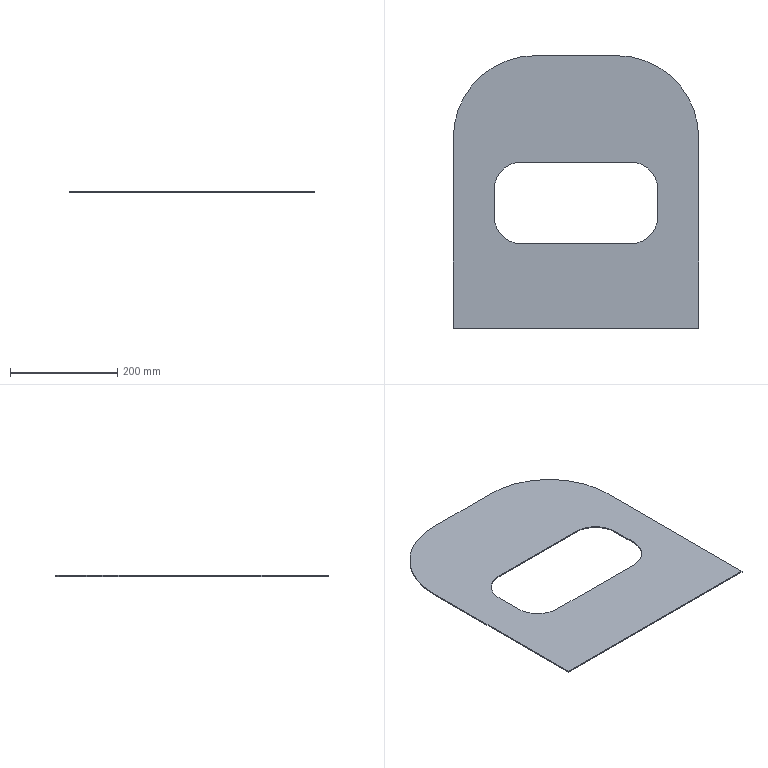Part | SolidWorks | features Extrusion 1 | 1 solid | 16 faces | box 457.2 x 508 x 2 mm | volume 356105 mm3 | plane 10 | cylinder 6 | commonest cylinder face diameters 101.6 x4 304.8 x2
STEP:
#1=CARTESIAN_POINT('',(228.6,0.,1.));
#2=VERTEX_POINT('',#1);
#3=CARTESIAN_POINT('',(228.6,355.6,1.));
#4=VERTEX_POINT('',#3);
#5=CARTESIAN_POINT('',(228.6,355.6,1.));
#6=DIRECTION('',(0.,1.,0.));
#7=VECTOR('',#6,1000.);
#8=LINE('',#5,#7);
#9=EDGE_CURVE('',#2,#4,#8,.T.);
#10=ORIENTED_EDGE('',*,*,#9,.T.);
#11=CARTESIAN_POINT('',(76.2,508.,1.));
#12=VERTEX_POINT('',#11);
#13=CARTESIAN_POINT('',(76.2,355.6,1.));
#14=DIRECTION('',(0.,0.,1.));
#15=DIRECTION('',(-1.,0.,0.));
#16=AXIS2_PLACEMENT_3D('',#13,#14,#15);
#17=CIRCLE('',#16,152.4);
#18=EDGE_CURVE('',#4,#12,#17,.T.);
#19=ORIENTED_EDGE('',*,*,#18,.T.);
#20=CARTESIAN_POINT('',(-76.2,508.,1.));
#21=VERTEX_POINT('',#20);
#22=CARTESIAN_POINT('',(-76.2,508.,1.));
#23=DIRECTION('',(-1.,0.,0.));
#24=VECTOR('',#23,1000.);
#25=LINE('',#22,#24);
#26=EDGE_CURVE('',#12,#21,#25,.T.);
#27=ORIENTED_EDGE('',*,*,#26,.T.);
#28=CARTESIAN_POINT('',(-228.6,355.6,1.));
#29=VERTEX_POINT('',#28);
#30=CARTESIAN_POINT('',(-76.2,355.6,1.));
#31=DIRECTION('',(0.,0.,1.));
#32=DIRECTION('',(1.,0.,0.));
#33=AXIS2_PLACEMENT_3D('',#30,#31,#32);
#34=CIRCLE('',#33,152.4);
#35=EDGE_CURVE('',#21,#29,#34,.T.);
#36=ORIENTED_EDGE('',*,*,#35,.T.);
#37=CARTESIAN_POINT('',(-228.6,0.,1.));
#38=VERTEX_POINT('',#37);
#39=CARTESIAN_POINT('',(-228.6,355.6,1.));
#40=DIRECTION('',(0.,-1.,0.));
#41=VECTOR('',#40,1000.);
#42=LINE('',#39,#41);
#43=EDGE_CURVE('',#29,#38,#42,.T.);
#44=ORIENTED_EDGE('',*,*,#43,.T.);
#45=CARTESIAN_POINT('',(-228.6,0.,1.));
#46=DIRECTION('',(1.,0.,0.));
#47=VECTOR('',#46,1000.);
#48=LINE('',#45,#47);
#49=EDGE_CURVE('',#38,#2,#48,.T.);
#50=ORIENTED_EDGE('',*,*,#49,.T.);
#51=EDGE_LOOP('',(#10,#19,#27,#36,#44,#50));
#52=FACE_OUTER_BOUND('',#51,.T.);
#53=CARTESIAN_POINT('',(101.6,309.88,1.));
#54=VERTEX_POINT('',#53);
#55=CARTESIAN_POINT('',(-101.6,309.88,1.));
#56=VERTEX_POINT('',#55);
#57=CARTESIAN_POINT('',(-101.6,309.88,1.));
#58=DIRECTION('',(-1.,0.,0.));
#59=VECTOR('',#58,1000.);
#60=LINE('',#57,#59);
#61=EDGE_CURVE('',#54,#56,#60,.T.);
#62=ORIENTED_EDGE('',*,*,#61,.F.);
#63=CARTESIAN_POINT('',(152.4,259.08,1.));
#64=VERTEX_POINT('',#63);
#65=CARTESIAN_POINT('',(101.6,259.08,1.));
#66=DIRECTION('',(0.,0.,1.));
#67=DIRECTION('',(-1.,0.,0.));
#68=AXIS2_PLACEMENT_3D('',#65,#66,#67);
#69=CIRCLE('',#68,50.8);
#70=EDGE_CURVE('',#64,#54,#69,.T.);
#71=ORIENTED_EDGE('',*,*,#70,.F.);
#72=CARTESIAN_POINT('',(152.4,208.28,1.));
#73=VERTEX_POINT('',#72);
#74=CARTESIAN_POINT('',(152.4,259.08,1.));
#75=DIRECTION('',(0.,1.,0.));
#76=VECTOR('',#75,1000.);
#77=LINE('',#74,#76);
#78=EDGE_CURVE('',#73,#64,#77,.T.);
#79=ORIENTED_EDGE('',*,*,#78,.F.);
#80=CARTESIAN_POINT('',(101.6,157.48,1.));
#81=VERTEX_POINT('',#80);
#82=CARTESIAN_POINT('',(101.6,208.28,1.));
#83=DIRECTION('',(0.,0.,1.));
#84=DIRECTION('',(1.,0.,0.));
#85=AXIS2_PLACEMENT_3D('',#82,#83,#84);
#86=CIRCLE('',#85,50.8);
#87=EDGE_CURVE('',#81,#73,#86,.T.);
#88=ORIENTED_EDGE('',*,*,#87,.F.);
#89=CARTESIAN_POINT('',(-101.6,157.48,1.));
#90=VERTEX_POINT('',#89);
#91=CARTESIAN_POINT('',(-101.6,157.48,1.));
#92=DIRECTION('',(1.,0.,0.));
#93=VECTOR('',#92,1000.);
#94=LINE('',#91,#93);
#95=EDGE_CURVE('',#90,#81,#94,.T.);
#96=ORIENTED_EDGE('',*,*,#95,.F.);
#97=CARTESIAN_POINT('',(-152.4,208.28,1.));
#98=VERTEX_POINT('',#97);
#99=CARTESIAN_POINT('',(-101.6,208.28,1.));
#100=DIRECTION('',(0.,0.,1.));
#101=DIRECTION('',(1.,0.,0.));
#102=AXIS2_PLACEMENT_3D('',#99,#100,#101);
#103=CIRCLE('',#102,50.8);
#104=EDGE_CURVE('',#98,#90,#103,.T.);
#105=ORIENTED_EDGE('',*,*,#104,.F.);
#106=CARTESIAN_POINT('',(-152.4,259.08,1.));
#107=VERTEX_POINT('',#106);
#108=CARTESIAN_POINT('',(-152.4,259.08,1.));
#109=DIRECTION('',(0.,-1.,0.));
#110=VECTOR('',#109,1000.);
#111=LINE('',#108,#110);
#112=EDGE_CURVE('',#107,#98,#111,.T.);
#113=ORIENTED_EDGE('',*,*,#112,.F.);
#114=CARTESIAN_POINT('',(-101.6,259.08,1.));
#115=DIRECTION('',(0.,0.,1.));
#116=DIRECTION('',(1.,0.,0.));
#117=AXIS2_PLACEMENT_3D('',#114,#115,#116);
#118=CIRCLE('',#117,50.8);
#119=EDGE_CURVE('',#56,#107,#118,.T.);
#120=ORIENTED_EDGE('',*,*,#119,.F.);
#121=EDGE_LOOP('',(#62,#71,#79,#88,#96,#105,#113,#120));
#122=FACE_BOUND('',#121,.T.);
#123=CARTESIAN_POINT('',(-76.2,355.6,1.));
#124=DIRECTION('',(0.,0.,1.));
#125=DIRECTION('',(1.,0.,0.));
#126=AXIS2_PLACEMENT_3D('',#123,#124,#125);
#127=PLANE('',#126);
#128=ADVANCED_FACE('',(#52,#122),#127,.T.);
#129=CARTESIAN_POINT('',(228.6,0.,-1.));
#130=VERTEX_POINT('',#129);
#131=CARTESIAN_POINT('',(228.6,355.6,-1.));
#132=VERTEX_POINT('',#131);
#133=CARTESIAN_POINT('',(228.6,355.6,-1.));
#134=DIRECTION('',(0.,1.,0.));
#135=VECTOR('',#134,1000.);
#136=LINE('',#133,#135);
#137=EDGE_CURVE('',#130,#132,#136,.T.);
#138=ORIENTED_EDGE('',*,*,#137,.F.);
#139=CARTESIAN_POINT('',(-228.6,0.,-1.));
#140=VERTEX_POINT('',#139);
#141=CARTESIAN_POINT('',(-228.6,0.,-1.));
#142=DIRECTION('',(1.,0.,0.));
#143=VECTOR('',#142,1000.);
#144=LINE('',#141,#143);
#145=EDGE_CURVE('',#140,#130,#144,.T.);
#146=ORIENTED_EDGE('',*,*,#145,.F.);
#147=CARTESIAN_POINT('',(-228.6,355.6,-1.));
#148=VERTEX_POINT('',#147);
#149=CARTESIAN_POINT('',(-228.6,355.6,-1.));
#150=DIRECTION('',(0.,-1.,0.));
#151=VECTOR('',#150,1000.);
#152=LINE('',#149,#151);
#153=EDGE_CURVE('',#148,#140,#152,.T.);
#154=ORIENTED_EDGE('',*,*,#153,.F.);
#155=CARTESIAN_POINT('',(-76.2,508.,-1.));
#156=VERTEX_POINT('',#155);
#157=CARTESIAN_POINT('',(-76.2,355.6,-1.));
#158=DIRECTION('',(0.,0.,1.));
#159=DIRECTION('',(1.,0.,0.));
#160=AXIS2_PLACEMENT_3D('',#157,#158,#159);
#161=CIRCLE('',#160,152.4);
#162=EDGE_CURVE('',#156,#148,#161,.T.);
#163=ORIENTED_EDGE('',*,*,#162,.F.);
#164=CARTESIAN_POINT('',(76.2,508.,-1.));
#165=VERTEX_POINT('',#164);
#166=CARTESIAN_POINT('',(-76.2,508.,-1.));
#167=DIRECTION('',(-1.,0.,0.));
#168=VECTOR('',#167,1000.);
#169=LINE('',#166,#168);
#170=EDGE_CURVE('',#165,#156,#169,.T.);
#171=ORIENTED_EDGE('',*,*,#170,.F.);
#172=CARTESIAN_POINT('',(76.2,355.6,-1.));
#173=DIRECTION('',(0.,0.,1.));
#174=DIRECTION('',(-1.,0.,0.));
#175=AXIS2_PLACEMENT_3D('',#172,#173,#174);
#176=CIRCLE('',#175,152.4);
#177=EDGE_CURVE('',#132,#165,#176,.T.);
#178=ORIENTED_EDGE('',*,*,#177,.F.);
#179=EDGE_LOOP('',(#138,#146,#154,#163,#171,#178));
#180=FACE_OUTER_BOUND('',#179,.T.);
#181=CARTESIAN_POINT('',(152.4,259.08,-1.));
#182=VERTEX_POINT('',#181);
#183=CARTESIAN_POINT('',(101.6,309.88,-1.));
#184=VERTEX_POINT('',#183);
#185=CARTESIAN_POINT('',(101.6,259.08,-1.));
#186=DIRECTION('',(0.,0.,1.));
#187=DIRECTION('',(-1.,0.,0.));
#188=AXIS2_PLACEMENT_3D('',#185,#186,#187);
#189=CIRCLE('',#188,50.8);
#190=EDGE_CURVE('',#182,#184,#189,.T.);
#191=ORIENTED_EDGE('',*,*,#190,.T.);
#192=CARTESIAN_POINT('',(-101.6,309.88,-1.));
#193=VERTEX_POINT('',#192);
#194=CARTESIAN_POINT('',(-101.6,309.88,-1.));
#195=DIRECTION('',(-1.,0.,0.));
#196=VECTOR('',#195,1000.);
#197=LINE('',#194,#196);
#198=EDGE_CURVE('',#184,#193,#197,.T.);
#199=ORIENTED_EDGE('',*,*,#198,.T.);
#200=CARTESIAN_POINT('',(-152.4,259.08,-1.));
#201=VERTEX_POINT('',#200);
#202=CARTESIAN_POINT('',(-101.6,259.08,-1.));
#203=DIRECTION('',(0.,0.,1.));
#204=DIRECTION('',(1.,0.,0.));
#205=AXIS2_PLACEMENT_3D('',#202,#203,#204);
#206=CIRCLE('',#205,50.8);
#207=EDGE_CURVE('',#193,#201,#206,.T.);
#208=ORIENTED_EDGE('',*,*,#207,.T.);
#209=CARTESIAN_POINT('',(-152.4,208.28,-1.));
#210=VERTEX_POINT('',#209);
#211=CARTESIAN_POINT('',(-152.4,259.08,-1.));
#212=DIRECTION('',(0.,-1.,0.));
#213=VECTOR('',#212,1000.);
#214=LINE('',#211,#213);
#215=EDGE_CURVE('',#201,#210,#214,.T.);
#216=ORIENTED_EDGE('',*,*,#215,.T.);
#217=CARTESIAN_POINT('',(-101.6,157.48,-1.));
#218=VERTEX_POINT('',#217);
#219=CARTESIAN_POINT('',(-101.6,208.28,-1.));
#220=DIRECTION('',(0.,0.,1.));
#221=DIRECTION('',(1.,0.,0.));
#222=AXIS2_PLACEMENT_3D('',#219,#220,#221);
#223=CIRCLE('',#222,50.8);
#224=EDGE_CURVE('',#210,#218,#223,.T.);
#225=ORIENTED_EDGE('',*,*,#224,.T.);
#226=CARTESIAN_POINT('',(101.6,157.48,-1.));
#227=VERTEX_POINT('',#226);
#228=CARTESIAN_POINT('',(-101.6,157.48,-1.));
#229=DIRECTION('',(1.,0.,0.));
#230=VECTOR('',#229,1000.);
#231=LINE('',#228,#230);
#232=EDGE_CURVE('',#218,#227,#231,.T.);
#233=ORIENTED_EDGE('',*,*,#232,.T.);
#234=CARTESIAN_POINT('',(152.4,208.28,-1.));
#235=VERTEX_POINT('',#234);
#236=CARTESIAN_POINT('',(101.6,208.28,-1.));
#237=DIRECTION('',(0.,0.,1.));
#238=DIRECTION('',(1.,0.,0.));
#239=AXIS2_PLACEMENT_3D('',#236,#237,#238);
#240=CIRCLE('',#239,50.8);
#241=EDGE_CURVE('',#227,#235,#240,.T.);
#242=ORIENTED_EDGE('',*,*,#241,.T.);
#243=CARTESIAN_POINT('',(152.4,259.08,-1.));
#244=DIRECTION('',(0.,1.,0.));
#245=VECTOR('',#244,1000.);
#246=LINE('',#243,#245);
#247=EDGE_CURVE('',#235,#182,#246,.T.);
#248=ORIENTED_EDGE('',*,*,#247,.T.);
#249=EDGE_LOOP('',(#191,#199,#208,#216,#225,#233,#242,#248));
#250=FACE_BOUND('',#249,.T.);
#251=CARTESIAN_POINT('',(-76.2,355.6,-1.));
#252=DIRECTION('',(0.,0.,1.));
#253=DIRECTION('',(1.,0.,0.));
#254=AXIS2_PLACEMENT_3D('',#251,#252,#253);
#255=PLANE('',#254);
#256=ADVANCED_FACE('',(#180,#250),#255,.F.);
#257=ORIENTED_EDGE('',*,*,#137,.T.);
#258=CARTESIAN_POINT('',(228.6,355.6,1.));
#259=DIRECTION('',(0.,0.,-1.));
#260=VECTOR('',#259,1000.);
#261=LINE('',#258,#260);
#262=EDGE_CURVE('',#4,#132,#261,.T.);
#263=ORIENTED_EDGE('',*,*,#262,.F.);
#264=ORIENTED_EDGE('',*,*,#9,.F.);
#265=CARTESIAN_POINT('',(228.6,0.,1.));
#266=DIRECTION('',(0.,0.,-1.));
#267=VECTOR('',#266,1000.);
#268=LINE('',#265,#267);
#269=EDGE_CURVE('',#2,#130,#268,.T.);
#270=ORIENTED_EDGE('',*,*,#269,.T.);
#271=EDGE_LOOP('',(#257,#263,#264,#270));
#272=FACE_OUTER_BOUND('',#271,.T.);
#273=CARTESIAN_POINT('',(228.6,355.6,1.));
#274=DIRECTION('',(-1.,0.,0.));
#275=DIRECTION('',(0.,-1.,0.));
#276=AXIS2_PLACEMENT_3D('',#273,#274,#275);
#277=PLANE('',#276);
#278=ADVANCED_FACE('',(#272),#277,.F.);
#279=ORIENTED_EDGE('',*,*,#177,.T.);
#280=CARTESIAN_POINT('',(76.2,508.,1.));
#281=DIRECTION('',(0.,0.,-1.));
#282=VECTOR('',#281,1000.);
#283=LINE('',#280,#282);
#284=EDGE_CURVE('',#12,#165,#283,.T.);
#285=ORIENTED_EDGE('',*,*,#284,.F.);
#286=ORIENTED_EDGE('',*,*,#18,.F.);
#287=ORIENTED_EDGE('',*,*,#262,.T.);
#288=EDGE_LOOP('',(#279,#285,#286,#287));
#289=FACE_OUTER_BOUND('',#288,.T.);
#290=CARTESIAN_POINT('',(76.2,355.6,1.));
#291=DIRECTION('',(0.,0.,-1.));
#292=DIRECTION('',(-1.,0.,0.));
#293=AXIS2_PLACEMENT_3D('',#290,#291,#292);
#294=CYLINDRICAL_SURFACE('',#293,152.4);
#295=ADVANCED_FACE('',(#289),#294,.T.);
#296=ORIENTED_EDGE('',*,*,#170,.T.);
#297=CARTESIAN_POINT('',(-76.2,508.,1.));
#298=DIRECTION('',(0.,0.,-1.));
#299=VECTOR('',#298,1000.);
#300=LINE('',#297,#299);
#301=EDGE_CURVE('',#21,#156,#300,.T.);
#302=ORIENTED_EDGE('',*,*,#301,.F.);
#303=ORIENTED_EDGE('',*,*,#26,.F.);
#304=ORIENTED_EDGE('',*,*,#284,.T.);
#305=EDGE_LOOP('',(#296,#302,#303,#304));
#306=FACE_OUTER_BOUND('',#305,.T.);
#307=CARTESIAN_POINT('',(-76.2,508.,1.));
#308=DIRECTION('',(0.,-1.,0.));
#309=DIRECTION('',(0.,0.,-1.));
#310=AXIS2_PLACEMENT_3D('',#307,#308,#309);
#311=PLANE('',#310);
#312=ADVANCED_FACE('',(#306),#311,.F.);
#313=ORIENTED_EDGE('',*,*,#162,.T.);
#314=CARTESIAN_POINT('',(-228.6,355.6,1.));
#315=DIRECTION('',(0.,0.,-1.));
#316=VECTOR('',#315,1000.);
#317=LINE('',#314,#316);
#318=EDGE_CURVE('',#29,#148,#317,.T.);
#319=ORIENTED_EDGE('',*,*,#318,.F.);
#320=ORIENTED_EDGE('',*,*,#35,.F.);
#321=ORIENTED_EDGE('',*,*,#301,.T.);
#322=EDGE_LOOP('',(#313,#319,#320,#321));
#323=FACE_OUTER_BOUND('',#322,.T.);
#324=CARTESIAN_POINT('',(-76.2,355.6,1.));
#325=DIRECTION('',(0.,0.,-1.));
#326=DIRECTION('',(-1.,0.,0.));
#327=AXIS2_PLACEMENT_3D('',#324,#325,#326);
#328=CYLINDRICAL_SURFACE('',#327,152.4);
#329=ADVANCED_FACE('',(#323),#328,.T.);
#330=ORIENTED_EDGE('',*,*,#153,.T.);
#331=CARTESIAN_POINT('',(-228.6,0.,1.));
#332=DIRECTION('',(0.,0.,-1.));
#333=VECTOR('',#332,1000.);
#334=LINE('',#331,#333);
#335=EDGE_CURVE('',#38,#140,#334,.T.);
#336=ORIENTED_EDGE('',*,*,#335,.F.);
#337=ORIENTED_EDGE('',*,*,#43,.F.);
#338=ORIENTED_EDGE('',*,*,#318,.T.);
#339=EDGE_LOOP('',(#330,#336,#337,#338));
#340=FACE_OUTER_BOUND('',#339,.T.);
#341=CARTESIAN_POINT('',(-228.6,355.6,1.));
#342=DIRECTION('',(1.,0.,0.));
#343=DIRECTION('',(0.,1.,0.));
#344=AXIS2_PLACEMENT_3D('',#341,#342,#343);
#345=PLANE('',#344);
#346=ADVANCED_FACE('',(#340),#345,.F.);
#347=ORIENTED_EDGE('',*,*,#145,.T.);
#348=ORIENTED_EDGE('',*,*,#269,.F.);
#349=ORIENTED_EDGE('',*,*,#49,.F.);
#350=ORIENTED_EDGE('',*,*,#335,.T.);
#351=EDGE_LOOP('',(#347,#348,#349,#350));
#352=FACE_OUTER_BOUND('',#351,.T.);
#353=CARTESIAN_POINT('',(-228.6,0.,1.));
#354=DIRECTION('',(0.,1.,0.));
#355=DIRECTION('',(-1.,0.,0.));
#356=AXIS2_PLACEMENT_3D('',#353,#354,#355);
#357=PLANE('',#356);
#358=ADVANCED_FACE('',(#352),#357,.F.);
#359=ORIENTED_EDGE('',*,*,#190,.F.);
#360=CARTESIAN_POINT('',(152.4,259.08,1.));
#361=DIRECTION('',(0.,0.,-1.));
#362=VECTOR('',#361,1000.);
#363=LINE('',#360,#362);
#364=EDGE_CURVE('',#64,#182,#363,.T.);
#365=ORIENTED_EDGE('',*,*,#364,.F.);
#366=ORIENTED_EDGE('',*,*,#70,.T.);
#367=CARTESIAN_POINT('',(101.6,309.88,1.));
#368=DIRECTION('',(0.,0.,-1.));
#369=VECTOR('',#368,1000.);
#370=LINE('',#367,#369);
#371=EDGE_CURVE('',#54,#184,#370,.T.);
#372=ORIENTED_EDGE('',*,*,#371,.T.);
#373=EDGE_LOOP('',(#359,#365,#366,#372));
#374=FACE_OUTER_BOUND('',#373,.T.);
#375=CARTESIAN_POINT('',(101.6,259.08,1.));
#376=DIRECTION('',(0.,0.,-1.));
#377=DIRECTION('',(-1.,0.,0.));
#378=AXIS2_PLACEMENT_3D('',#375,#376,#377);
#379=CYLINDRICAL_SURFACE('',#378,50.8);
#380=ADVANCED_FACE('',(#374),#379,.F.);
#381=ORIENTED_EDGE('',*,*,#198,.F.);
#382=ORIENTED_EDGE('',*,*,#371,.F.);
#383=ORIENTED_EDGE('',*,*,#61,.T.);
#384=CARTESIAN_POINT('',(-101.6,309.88,1.));
#385=DIRECTION('',(0.,0.,-1.));
#386=VECTOR('',#385,1000.);
#387=LINE('',#384,#386);
#388=EDGE_CURVE('',#56,#193,#387,.T.);
#389=ORIENTED_EDGE('',*,*,#388,.T.);
#390=EDGE_LOOP('',(#381,#382,#383,#389));
#391=FACE_OUTER_BOUND('',#390,.T.);
#392=CARTESIAN_POINT('',(-101.6,309.88,1.));
#393=DIRECTION('',(0.,-1.,0.));
#394=DIRECTION('',(1.,0.,0.));
#395=AXIS2_PLACEMENT_3D('',#392,#393,#394);
#396=PLANE('',#395);
#397=ADVANCED_FACE('',(#391),#396,.T.);
#398=ORIENTED_EDGE('',*,*,#207,.F.);
#399=ORIENTED_EDGE('',*,*,#388,.F.);
#400=ORIENTED_EDGE('',*,*,#119,.T.);
#401=CARTESIAN_POINT('',(-152.4,259.08,1.));
#402=DIRECTION('',(0.,0.,-1.));
#403=VECTOR('',#402,1000.);
#404=LINE('',#401,#403);
#405=EDGE_CURVE('',#107,#201,#404,.T.);
#406=ORIENTED_EDGE('',*,*,#405,.T.);
#407=EDGE_LOOP('',(#398,#399,#400,#406));
#408=FACE_OUTER_BOUND('',#407,.T.);
#409=CARTESIAN_POINT('',(-101.6,259.08,1.));
#410=DIRECTION('',(0.,0.,-1.));
#411=DIRECTION('',(-1.,0.,0.));
#412=AXIS2_PLACEMENT_3D('',#409,#410,#411);
#413=CYLINDRICAL_SURFACE('',#412,50.8);
#414=ADVANCED_FACE('',(#408),#413,.F.);
#415=ORIENTED_EDGE('',*,*,#215,.F.);
#416=ORIENTED_EDGE('',*,*,#405,.F.);
#417=ORIENTED_EDGE('',*,*,#112,.T.);
#418=CARTESIAN_POINT('',(-152.4,208.28,1.));
#419=DIRECTION('',(0.,0.,-1.));
#420=VECTOR('',#419,1000.);
#421=LINE('',#418,#420);
#422=EDGE_CURVE('',#98,#210,#421,.T.);
#423=ORIENTED_EDGE('',*,*,#422,.T.);
#424=EDGE_LOOP('',(#415,#416,#417,#423));
#425=FACE_OUTER_BOUND('',#424,.T.);
#426=CARTESIAN_POINT('',(-152.4,259.08,1.));
#427=DIRECTION('',(1.,0.,0.));
#428=DIRECTION('',(0.,0.,-1.));
#429=AXIS2_PLACEMENT_3D('',#426,#427,#428);
#430=PLANE('',#429);
#431=ADVANCED_FACE('',(#425),#430,.T.);
#432=ORIENTED_EDGE('',*,*,#224,.F.);
#433=ORIENTED_EDGE('',*,*,#422,.F.);
#434=ORIENTED_EDGE('',*,*,#104,.T.);
#435=CARTESIAN_POINT('',(-101.6,157.48,1.));
#436=DIRECTION('',(0.,0.,-1.));
#437=VECTOR('',#436,1000.);
#438=LINE('',#435,#437);
#439=EDGE_CURVE('',#90,#218,#438,.T.);
#440=ORIENTED_EDGE('',*,*,#439,.T.);
#441=EDGE_LOOP('',(#432,#433,#434,#440));
#442=FACE_OUTER_BOUND('',#441,.T.);
#443=CARTESIAN_POINT('',(-101.6,208.28,1.));
#444=DIRECTION('',(0.,0.,-1.));
#445=DIRECTION('',(-1.,0.,0.));
#446=AXIS2_PLACEMENT_3D('',#443,#444,#445);
#447=CYLINDRICAL_SURFACE('',#446,50.8);
#448=ADVANCED_FACE('',(#442),#447,.F.);
#449=ORIENTED_EDGE('',*,*,#232,.F.);
#450=ORIENTED_EDGE('',*,*,#439,.F.);
#451=ORIENTED_EDGE('',*,*,#95,.T.);
#452=CARTESIAN_POINT('',(101.6,157.48,1.));
#453=DIRECTION('',(0.,0.,-1.));
#454=VECTOR('',#453,1000.);
#455=LINE('',#452,#454);
#456=EDGE_CURVE('',#81,#227,#455,.T.);
#457=ORIENTED_EDGE('',*,*,#456,.T.);
#458=EDGE_LOOP('',(#449,#450,#451,#457));
#459=FACE_OUTER_BOUND('',#458,.T.);
#460=CARTESIAN_POINT('',(-101.6,157.48,1.));
#461=DIRECTION('',(0.,1.,0.));
#462=DIRECTION('',(-1.,0.,0.));
#463=AXIS2_PLACEMENT_3D('',#460,#461,#462);
#464=PLANE('',#463);
#465=ADVANCED_FACE('',(#459),#464,.T.);
#466=ORIENTED_EDGE('',*,*,#241,.F.);
#467=ORIENTED_EDGE('',*,*,#456,.F.);
#468=ORIENTED_EDGE('',*,*,#87,.T.);
#469=CARTESIAN_POINT('',(152.4,208.28,1.));
#470=DIRECTION('',(0.,0.,-1.));
#471=VECTOR('',#470,1000.);
#472=LINE('',#469,#471);
#473=EDGE_CURVE('',#73,#235,#472,.T.);
#474=ORIENTED_EDGE('',*,*,#473,.T.);
#475=EDGE_LOOP('',(#466,#467,#468,#474));
#476=FACE_OUTER_BOUND('',#475,.T.);
#477=CARTESIAN_POINT('',(101.6,208.28,1.));
#478=DIRECTION('',(0.,0.,-1.));
#479=DIRECTION('',(-1.,0.,0.));
#480=AXIS2_PLACEMENT_3D('',#477,#478,#479);
#481=CYLINDRICAL_SURFACE('',#480,50.8);
#482=ADVANCED_FACE('',(#476),#481,.F.);
#483=ORIENTED_EDGE('',*,*,#247,.F.);
#484=ORIENTED_EDGE('',*,*,#473,.F.);
#485=ORIENTED_EDGE('',*,*,#78,.T.);
#486=ORIENTED_EDGE('',*,*,#364,.T.);
#487=EDGE_LOOP('',(#483,#484,#485,#486));
#488=FACE_OUTER_BOUND('',#487,.T.);
#489=CARTESIAN_POINT('',(152.4,259.08,1.));
#490=DIRECTION('',(-1.,0.,0.));
#491=DIRECTION('',(0.,0.,1.));
#492=AXIS2_PLACEMENT_3D('',#489,#490,#491);
#493=PLANE('',#492);
#494=ADVANCED_FACE('',(#488),#493,.T.);
#495=CLOSED_SHELL('',(#128,#256,#278,#295,#312,#329,#346,#358,#380,#397,#414,#431,#448,#465,#482,#494));
#496=MANIFOLD_SOLID_BREP('',#495);
#497=CARTESIAN_POINT('',(0.,0.,0.));
#498=DIRECTION('',(0.,0.,1.));
#499=DIRECTION('',(1.,0.,0.));
#500=AXIS2_PLACEMENT_3D('',#497,#498,#499);
#501=(LENGTH_UNIT()NAMED_UNIT(*)SI_UNIT(.MILLI.,.METRE.));
#502=UNCERTAINTY_MEASURE_WITH_UNIT(LENGTH_MEASURE(0.00001),#501,'','');
#503=(NAMED_UNIT(*)PLANE_ANGLE_UNIT()SI_UNIT($,.RADIAN.));
#504=(NAMED_UNIT(*)SI_UNIT($,.STERADIAN.)SOLID_ANGLE_UNIT());
#505=(GEOMETRIC_REPRESENTATION_CONTEXT(3)GLOBAL_UNCERTAINTY_ASSIGNED_CONTEXT((#502))GLOBAL_UNIT_ASSIGNED_CONTEXT((#501,#503,#504))REPRESENTATION_CONTEXT('',''));
#506=ADVANCED_BREP_SHAPE_REPRESENTATION('',(#496,#500),#505);